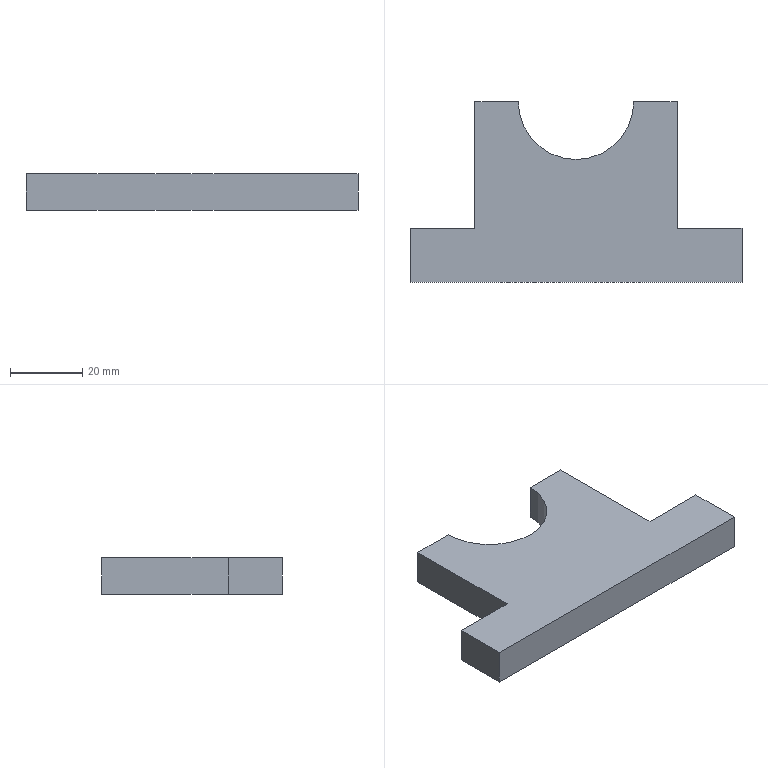Part | SolidWorks | features Extrusion 1 | 1 solid | 12 faces | box 92 x 50 x 10 mm | volume 29379 mm3 | plane 11 | cylinder 1 | commonest cylinder face diameters 32 x1
STEP:
#1=CARTESIAN_POINT('',(16.,50.,0.));
#2=VERTEX_POINT('',#1);
#3=CARTESIAN_POINT('',(-16.,50.,0.));
#4=VERTEX_POINT('',#3);
#5=CARTESIAN_POINT('',(0.,50.,0.));
#6=DIRECTION('',(0.,0.,-1.));
#7=DIRECTION('',(1.,0.,0.));
#8=AXIS2_PLACEMENT_3D('',#5,#6,#7);
#9=CIRCLE('',#8,16.);
#10=EDGE_CURVE('',#2,#4,#9,.T.);
#11=ORIENTED_EDGE('',*,*,#10,.T.);
#12=CARTESIAN_POINT('',(-16.,50.,10.));
#13=VERTEX_POINT('',#12);
#14=CARTESIAN_POINT('',(-16.,50.,10.));
#15=DIRECTION('',(0.,0.,-1.));
#16=VECTOR('',#15,1000.);
#17=LINE('',#14,#16);
#18=EDGE_CURVE('',#13,#4,#17,.T.);
#19=ORIENTED_EDGE('',*,*,#18,.F.);
#20=CARTESIAN_POINT('',(16.,50.,10.));
#21=VERTEX_POINT('',#20);
#22=CARTESIAN_POINT('',(0.,50.,10.));
#23=DIRECTION('',(0.,0.,-1.));
#24=DIRECTION('',(1.,0.,0.));
#25=AXIS2_PLACEMENT_3D('',#22,#23,#24);
#26=CIRCLE('',#25,16.);
#27=EDGE_CURVE('',#21,#13,#26,.T.);
#28=ORIENTED_EDGE('',*,*,#27,.F.);
#29=CARTESIAN_POINT('',(16.,50.,10.));
#30=DIRECTION('',(0.,0.,-1.));
#31=VECTOR('',#30,1000.);
#32=LINE('',#29,#31);
#33=EDGE_CURVE('',#21,#2,#32,.T.);
#34=ORIENTED_EDGE('',*,*,#33,.T.);
#35=EDGE_LOOP('',(#11,#19,#28,#34));
#36=FACE_OUTER_BOUND('',#35,.T.);
#37=CARTESIAN_POINT('',(0.,50.,10.));
#38=DIRECTION('',(0.,0.,-1.));
#39=DIRECTION('',(-1.,0.,0.));
#40=AXIS2_PLACEMENT_3D('',#37,#38,#39);
#41=CYLINDRICAL_SURFACE('',#40,16.);
#42=ADVANCED_FACE('',(#36),#41,.F.);
#43=CARTESIAN_POINT('',(-28.,50.,0.));
#44=VERTEX_POINT('',#43);
#45=CARTESIAN_POINT('',(-16.,50.,0.));
#46=DIRECTION('',(-1.,0.,0.));
#47=VECTOR('',#46,1000.);
#48=LINE('',#45,#47);
#49=EDGE_CURVE('',#4,#44,#48,.T.);
#50=ORIENTED_EDGE('',*,*,#49,.T.);
#51=CARTESIAN_POINT('',(-28.,50.,10.));
#52=VERTEX_POINT('',#51);
#53=CARTESIAN_POINT('',(-28.,50.,10.));
#54=DIRECTION('',(0.,0.,-1.));
#55=VECTOR('',#54,1000.);
#56=LINE('',#53,#55);
#57=EDGE_CURVE('',#52,#44,#56,.T.);
#58=ORIENTED_EDGE('',*,*,#57,.F.);
#59=CARTESIAN_POINT('',(-16.,50.,10.));
#60=DIRECTION('',(-1.,0.,0.));
#61=VECTOR('',#60,1000.);
#62=LINE('',#59,#61);
#63=EDGE_CURVE('',#13,#52,#62,.T.);
#64=ORIENTED_EDGE('',*,*,#63,.F.);
#65=ORIENTED_EDGE('',*,*,#18,.T.);
#66=EDGE_LOOP('',(#50,#58,#64,#65));
#67=FACE_OUTER_BOUND('',#66,.T.);
#68=CARTESIAN_POINT('',(-16.,50.,10.));
#69=DIRECTION('',(0.,-1.,0.));
#70=DIRECTION('',(0.,0.,-1.));
#71=AXIS2_PLACEMENT_3D('',#68,#69,#70);
#72=PLANE('',#71);
#73=ADVANCED_FACE('',(#67),#72,.F.);
#74=CARTESIAN_POINT('',(-28.,15.,0.));
#75=VERTEX_POINT('',#74);
#76=CARTESIAN_POINT('',(-28.,50.,0.));
#77=DIRECTION('',(0.,-1.,0.));
#78=VECTOR('',#77,1000.);
#79=LINE('',#76,#78);
#80=EDGE_CURVE('',#44,#75,#79,.T.);
#81=ORIENTED_EDGE('',*,*,#80,.T.);
#82=CARTESIAN_POINT('',(-28.,15.,10.));
#83=VERTEX_POINT('',#82);
#84=CARTESIAN_POINT('',(-28.,15.,10.));
#85=DIRECTION('',(0.,0.,-1.));
#86=VECTOR('',#85,1000.);
#87=LINE('',#84,#86);
#88=EDGE_CURVE('',#83,#75,#87,.T.);
#89=ORIENTED_EDGE('',*,*,#88,.F.);
#90=CARTESIAN_POINT('',(-28.,50.,10.));
#91=DIRECTION('',(0.,-1.,0.));
#92=VECTOR('',#91,1000.);
#93=LINE('',#90,#92);
#94=EDGE_CURVE('',#52,#83,#93,.T.);
#95=ORIENTED_EDGE('',*,*,#94,.F.);
#96=ORIENTED_EDGE('',*,*,#57,.T.);
#97=EDGE_LOOP('',(#81,#89,#95,#96));
#98=FACE_OUTER_BOUND('',#97,.T.);
#99=CARTESIAN_POINT('',(-28.,50.,10.));
#100=DIRECTION('',(1.,0.,0.));
#101=DIRECTION('',(0.,1.,0.));
#102=AXIS2_PLACEMENT_3D('',#99,#100,#101);
#103=PLANE('',#102);
#104=ADVANCED_FACE('',(#98),#103,.F.);
#105=CARTESIAN_POINT('',(-46.,15.,0.));
#106=VERTEX_POINT('',#105);
#107=CARTESIAN_POINT('',(-28.,15.,0.));
#108=DIRECTION('',(-1.,0.,0.));
#109=VECTOR('',#108,1000.);
#110=LINE('',#107,#109);
#111=EDGE_CURVE('',#75,#106,#110,.T.);
#112=ORIENTED_EDGE('',*,*,#111,.T.);
#113=CARTESIAN_POINT('',(-46.,15.,10.));
#114=VERTEX_POINT('',#113);
#115=CARTESIAN_POINT('',(-46.,15.,10.));
#116=DIRECTION('',(0.,0.,-1.));
#117=VECTOR('',#116,1000.);
#118=LINE('',#115,#117);
#119=EDGE_CURVE('',#114,#106,#118,.T.);
#120=ORIENTED_EDGE('',*,*,#119,.F.);
#121=CARTESIAN_POINT('',(-28.,15.,10.));
#122=DIRECTION('',(-1.,0.,0.));
#123=VECTOR('',#122,1000.);
#124=LINE('',#121,#123);
#125=EDGE_CURVE('',#83,#114,#124,.T.);
#126=ORIENTED_EDGE('',*,*,#125,.F.);
#127=ORIENTED_EDGE('',*,*,#88,.T.);
#128=EDGE_LOOP('',(#112,#120,#126,#127));
#129=FACE_OUTER_BOUND('',#128,.T.);
#130=CARTESIAN_POINT('',(-28.,15.,10.));
#131=DIRECTION('',(0.,-1.,0.));
#132=DIRECTION('',(1.,0.,0.));
#133=AXIS2_PLACEMENT_3D('',#130,#131,#132);
#134=PLANE('',#133);
#135=ADVANCED_FACE('',(#129),#134,.F.);
#136=CARTESIAN_POINT('',(-46.,0.,0.));
#137=VERTEX_POINT('',#136);
#138=CARTESIAN_POINT('',(-46.,15.,0.));
#139=DIRECTION('',(0.,-1.,0.));
#140=VECTOR('',#139,1000.);
#141=LINE('',#138,#140);
#142=EDGE_CURVE('',#106,#137,#141,.T.);
#143=ORIENTED_EDGE('',*,*,#142,.T.);
#144=CARTESIAN_POINT('',(-46.,0.,10.));
#145=VERTEX_POINT('',#144);
#146=CARTESIAN_POINT('',(-46.,0.,10.));
#147=DIRECTION('',(0.,0.,-1.));
#148=VECTOR('',#147,1000.);
#149=LINE('',#146,#148);
#150=EDGE_CURVE('',#145,#137,#149,.T.);
#151=ORIENTED_EDGE('',*,*,#150,.F.);
#152=CARTESIAN_POINT('',(-46.,15.,10.));
#153=DIRECTION('',(0.,-1.,0.));
#154=VECTOR('',#153,1000.);
#155=LINE('',#152,#154);
#156=EDGE_CURVE('',#114,#145,#155,.T.);
#157=ORIENTED_EDGE('',*,*,#156,.F.);
#158=ORIENTED_EDGE('',*,*,#119,.T.);
#159=EDGE_LOOP('',(#143,#151,#157,#158));
#160=FACE_OUTER_BOUND('',#159,.T.);
#161=CARTESIAN_POINT('',(-46.,15.,10.));
#162=DIRECTION('',(1.,0.,0.));
#163=DIRECTION('',(0.,0.,-1.));
#164=AXIS2_PLACEMENT_3D('',#161,#162,#163);
#165=PLANE('',#164);
#166=ADVANCED_FACE('',(#160),#165,.F.);
#167=CARTESIAN_POINT('',(46.,0.,0.));
#168=VERTEX_POINT('',#167);
#169=CARTESIAN_POINT('',(-46.,0.,0.));
#170=DIRECTION('',(1.,0.,0.));
#171=VECTOR('',#170,1000.);
#172=LINE('',#169,#171);
#173=EDGE_CURVE('',#137,#168,#172,.T.);
#174=ORIENTED_EDGE('',*,*,#173,.T.);
#175=CARTESIAN_POINT('',(46.,0.,10.));
#176=VERTEX_POINT('',#175);
#177=CARTESIAN_POINT('',(46.,0.,10.));
#178=DIRECTION('',(0.,0.,-1.));
#179=VECTOR('',#178,1000.);
#180=LINE('',#177,#179);
#181=EDGE_CURVE('',#176,#168,#180,.T.);
#182=ORIENTED_EDGE('',*,*,#181,.F.);
#183=CARTESIAN_POINT('',(-46.,0.,10.));
#184=DIRECTION('',(1.,0.,0.));
#185=VECTOR('',#184,1000.);
#186=LINE('',#183,#185);
#187=EDGE_CURVE('',#145,#176,#186,.T.);
#188=ORIENTED_EDGE('',*,*,#187,.F.);
#189=ORIENTED_EDGE('',*,*,#150,.T.);
#190=EDGE_LOOP('',(#174,#182,#188,#189));
#191=FACE_OUTER_BOUND('',#190,.T.);
#192=CARTESIAN_POINT('',(-46.,0.,10.));
#193=DIRECTION('',(0.,1.,0.));
#194=DIRECTION('',(0.,0.,1.));
#195=AXIS2_PLACEMENT_3D('',#192,#193,#194);
#196=PLANE('',#195);
#197=ADVANCED_FACE('',(#191),#196,.F.);
#198=CARTESIAN_POINT('',(46.,15.,0.));
#199=VERTEX_POINT('',#198);
#200=CARTESIAN_POINT('',(46.,15.,0.));
#201=DIRECTION('',(0.,1.,0.));
#202=VECTOR('',#201,1000.);
#203=LINE('',#200,#202);
#204=EDGE_CURVE('',#168,#199,#203,.T.);
#205=ORIENTED_EDGE('',*,*,#204,.T.);
#206=CARTESIAN_POINT('',(46.,15.,10.));
#207=VERTEX_POINT('',#206);
#208=CARTESIAN_POINT('',(46.,15.,10.));
#209=DIRECTION('',(0.,0.,-1.));
#210=VECTOR('',#209,1000.);
#211=LINE('',#208,#210);
#212=EDGE_CURVE('',#207,#199,#211,.T.);
#213=ORIENTED_EDGE('',*,*,#212,.F.);
#214=CARTESIAN_POINT('',(46.,15.,10.));
#215=DIRECTION('',(0.,1.,0.));
#216=VECTOR('',#215,1000.);
#217=LINE('',#214,#216);
#218=EDGE_CURVE('',#176,#207,#217,.T.);
#219=ORIENTED_EDGE('',*,*,#218,.F.);
#220=ORIENTED_EDGE('',*,*,#181,.T.);
#221=EDGE_LOOP('',(#205,#213,#219,#220));
#222=FACE_OUTER_BOUND('',#221,.T.);
#223=CARTESIAN_POINT('',(46.,15.,10.));
#224=DIRECTION('',(-1.,0.,0.));
#225=DIRECTION('',(0.,0.,1.));
#226=AXIS2_PLACEMENT_3D('',#223,#224,#225);
#227=PLANE('',#226);
#228=ADVANCED_FACE('',(#222),#227,.F.);
#229=CARTESIAN_POINT('',(28.,15.,0.));
#230=VERTEX_POINT('',#229);
#231=CARTESIAN_POINT('',(28.,15.,0.));
#232=DIRECTION('',(-1.,0.,0.));
#233=VECTOR('',#232,1000.);
#234=LINE('',#231,#233);
#235=EDGE_CURVE('',#199,#230,#234,.T.);
#236=ORIENTED_EDGE('',*,*,#235,.T.);
#237=CARTESIAN_POINT('',(28.,15.,10.));
#238=VERTEX_POINT('',#237);
#239=CARTESIAN_POINT('',(28.,15.,10.));
#240=DIRECTION('',(0.,0.,-1.));
#241=VECTOR('',#240,1000.);
#242=LINE('',#239,#241);
#243=EDGE_CURVE('',#238,#230,#242,.T.);
#244=ORIENTED_EDGE('',*,*,#243,.F.);
#245=CARTESIAN_POINT('',(28.,15.,10.));
#246=DIRECTION('',(-1.,0.,0.));
#247=VECTOR('',#246,1000.);
#248=LINE('',#245,#247);
#249=EDGE_CURVE('',#207,#238,#248,.T.);
#250=ORIENTED_EDGE('',*,*,#249,.F.);
#251=ORIENTED_EDGE('',*,*,#212,.T.);
#252=EDGE_LOOP('',(#236,#244,#250,#251));
#253=FACE_OUTER_BOUND('',#252,.T.);
#254=CARTESIAN_POINT('',(28.,15.,10.));
#255=DIRECTION('',(0.,-1.,0.));
#256=DIRECTION('',(1.,0.,0.));
#257=AXIS2_PLACEMENT_3D('',#254,#255,#256);
#258=PLANE('',#257);
#259=ADVANCED_FACE('',(#253),#258,.F.);
#260=CARTESIAN_POINT('',(28.,50.,0.));
#261=VERTEX_POINT('',#260);
#262=CARTESIAN_POINT('',(28.,50.,0.));
#263=DIRECTION('',(0.,1.,0.));
#264=VECTOR('',#263,1000.);
#265=LINE('',#262,#264);
#266=EDGE_CURVE('',#230,#261,#265,.T.);
#267=ORIENTED_EDGE('',*,*,#266,.T.);
#268=CARTESIAN_POINT('',(28.,50.,10.));
#269=VERTEX_POINT('',#268);
#270=CARTESIAN_POINT('',(28.,50.,10.));
#271=DIRECTION('',(0.,0.,-1.));
#272=VECTOR('',#271,1000.);
#273=LINE('',#270,#272);
#274=EDGE_CURVE('',#269,#261,#273,.T.);
#275=ORIENTED_EDGE('',*,*,#274,.F.);
#276=CARTESIAN_POINT('',(28.,50.,10.));
#277=DIRECTION('',(0.,1.,0.));
#278=VECTOR('',#277,1000.);
#279=LINE('',#276,#278);
#280=EDGE_CURVE('',#238,#269,#279,.T.);
#281=ORIENTED_EDGE('',*,*,#280,.F.);
#282=ORIENTED_EDGE('',*,*,#243,.T.);
#283=EDGE_LOOP('',(#267,#275,#281,#282));
#284=FACE_OUTER_BOUND('',#283,.T.);
#285=CARTESIAN_POINT('',(28.,50.,10.));
#286=DIRECTION('',(-1.,0.,0.));
#287=DIRECTION('',(0.,-1.,0.));
#288=AXIS2_PLACEMENT_3D('',#285,#286,#287);
#289=PLANE('',#288);
#290=ADVANCED_FACE('',(#284),#289,.F.);
#291=CARTESIAN_POINT('',(16.,50.,0.));
#292=DIRECTION('',(-1.,0.,0.));
#293=VECTOR('',#292,1000.);
#294=LINE('',#291,#293);
#295=EDGE_CURVE('',#261,#2,#294,.T.);
#296=ORIENTED_EDGE('',*,*,#295,.T.);
#297=ORIENTED_EDGE('',*,*,#33,.F.);
#298=CARTESIAN_POINT('',(16.,50.,10.));
#299=DIRECTION('',(-1.,0.,0.));
#300=VECTOR('',#299,1000.);
#301=LINE('',#298,#300);
#302=EDGE_CURVE('',#269,#21,#301,.T.);
#303=ORIENTED_EDGE('',*,*,#302,.F.);
#304=ORIENTED_EDGE('',*,*,#274,.T.);
#305=EDGE_LOOP('',(#296,#297,#303,#304));
#306=FACE_OUTER_BOUND('',#305,.T.);
#307=CARTESIAN_POINT('',(16.,50.,10.));
#308=DIRECTION('',(0.,-1.,0.));
#309=DIRECTION('',(0.,0.,-1.));
#310=AXIS2_PLACEMENT_3D('',#307,#308,#309);
#311=PLANE('',#310);
#312=ADVANCED_FACE('',(#306),#311,.F.);
#313=ORIENTED_EDGE('',*,*,#27,.T.);
#314=ORIENTED_EDGE('',*,*,#63,.T.);
#315=ORIENTED_EDGE('',*,*,#94,.T.);
#316=ORIENTED_EDGE('',*,*,#125,.T.);
#317=ORIENTED_EDGE('',*,*,#156,.T.);
#318=ORIENTED_EDGE('',*,*,#187,.T.);
#319=ORIENTED_EDGE('',*,*,#218,.T.);
#320=ORIENTED_EDGE('',*,*,#249,.T.);
#321=ORIENTED_EDGE('',*,*,#280,.T.);
#322=ORIENTED_EDGE('',*,*,#302,.T.);
#323=EDGE_LOOP('',(#313,#314,#315,#316,#317,#318,#319,#320,#321,#322));
#324=FACE_OUTER_BOUND('',#323,.T.);
#325=CARTESIAN_POINT('',(0.,50.,10.));
#326=DIRECTION('',(0.,0.,1.));
#327=DIRECTION('',(1.,0.,0.));
#328=AXIS2_PLACEMENT_3D('',#325,#326,#327);
#329=PLANE('',#328);
#330=ADVANCED_FACE('',(#324),#329,.T.);
#331=ORIENTED_EDGE('',*,*,#10,.F.);
#332=ORIENTED_EDGE('',*,*,#295,.F.);
#333=ORIENTED_EDGE('',*,*,#266,.F.);
#334=ORIENTED_EDGE('',*,*,#235,.F.);
#335=ORIENTED_EDGE('',*,*,#204,.F.);
#336=ORIENTED_EDGE('',*,*,#173,.F.);
#337=ORIENTED_EDGE('',*,*,#142,.F.);
#338=ORIENTED_EDGE('',*,*,#111,.F.);
#339=ORIENTED_EDGE('',*,*,#80,.F.);
#340=ORIENTED_EDGE('',*,*,#49,.F.);
#341=EDGE_LOOP('',(#331,#332,#333,#334,#335,#336,#337,#338,#339,#340));
#342=FACE_OUTER_BOUND('',#341,.T.);
#343=CARTESIAN_POINT('',(0.,50.,0.));
#344=DIRECTION('',(0.,0.,1.));
#345=DIRECTION('',(1.,0.,0.));
#346=AXIS2_PLACEMENT_3D('',#343,#344,#345);
#347=PLANE('',#346);
#348=ADVANCED_FACE('',(#342),#347,.F.);
#349=CLOSED_SHELL('',(#42,#73,#104,#135,#166,#197,#228,#259,#290,#312,#330,#348));
#350=MANIFOLD_SOLID_BREP('',#349);
#351=CARTESIAN_POINT('',(0.,0.,0.));
#352=DIRECTION('',(0.,0.,1.));
#353=DIRECTION('',(1.,0.,0.));
#354=AXIS2_PLACEMENT_3D('',#351,#352,#353);
#355=(LENGTH_UNIT()NAMED_UNIT(*)SI_UNIT(.MILLI.,.METRE.));
#356=UNCERTAINTY_MEASURE_WITH_UNIT(LENGTH_MEASURE(0.00001),#355,'','');
#357=(NAMED_UNIT(*)PLANE_ANGLE_UNIT()SI_UNIT($,.RADIAN.));
#358=(NAMED_UNIT(*)SI_UNIT($,.STERADIAN.)SOLID_ANGLE_UNIT());
#359=(GEOMETRIC_REPRESENTATION_CONTEXT(3)GLOBAL_UNCERTAINTY_ASSIGNED_CONTEXT((#356))GLOBAL_UNIT_ASSIGNED_CONTEXT((#355,#357,#358))REPRESENTATION_CONTEXT('',''));
#360=ADVANCED_BREP_SHAPE_REPRESENTATION('',(#350,#354),#359);